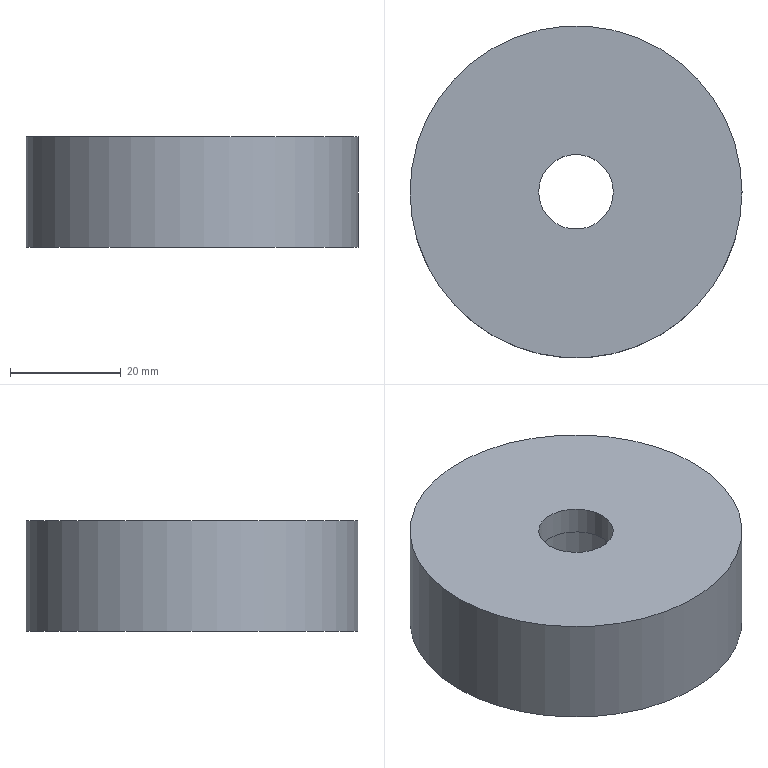Part | NX | features solid 2 | 1 solid | 6 faces | box 60 x 60 x 20 mm | volume 51121 mm3 | cylinder 3 | plane 3 | commonest cylinder face diameters 13.5 x1 20 x1 60 x1
STEP:
#1=CARTESIAN_POINT('',(-260.,-630.,220.));
#2=VERTEX_POINT('',#1);
#3=CARTESIAN_POINT('',(-290.,-630.,220.));
#4=DIRECTION('',(0.,0.,1.));
#5=DIRECTION('',(1.,0.,0.));
#6=AXIS2_PLACEMENT_3D('',#3,#4,#5);
#7=CIRCLE('',#6,30.);
#8=EDGE_CURVE('',#2,#2,#7,.T.);
#9=ORIENTED_EDGE('',*,*,#8,.T.);
#10=EDGE_LOOP('',(#9));
#11=FACE_BOUND('',#10,.T.);
#12=CARTESIAN_POINT('',(-260.,-630.,240.));
#13=VERTEX_POINT('',#12);
#14=CARTESIAN_POINT('',(-290.,-630.,240.));
#15=DIRECTION('',(0.,0.,1.));
#16=DIRECTION('',(1.,0.,0.));
#17=AXIS2_PLACEMENT_3D('',#14,#15,#16);
#18=CIRCLE('',#17,30.);
#19=EDGE_CURVE('',#13,#13,#18,.T.);
#20=ORIENTED_EDGE('',*,*,#19,.F.);
#21=EDGE_LOOP('',(#20));
#22=FACE_BOUND('',#21,.T.);
#23=CARTESIAN_POINT('',(-290.,-630.,220.));
#24=DIRECTION('',(0.,0.,1.));
#25=DIRECTION('',(-1.,0.,0.));
#26=AXIS2_PLACEMENT_3D('',#23,#24,#25);
#27=CYLINDRICAL_SURFACE('',#26,30.);
#28=ADVANCED_FACE('',(#11,#22),#27,.T.);
#29=CARTESIAN_POINT('',(-280.,-630.,220.));
#30=VERTEX_POINT('',#29);
#31=CARTESIAN_POINT('',(-290.,-630.,220.));
#32=DIRECTION('',(0.,0.,1.));
#33=DIRECTION('',(1.,0.,0.));
#34=AXIS2_PLACEMENT_3D('',#31,#32,#33);
#35=CIRCLE('',#34,10.);
#36=EDGE_CURVE('',#30,#30,#35,.T.);
#37=ORIENTED_EDGE('',*,*,#36,.T.);
#38=EDGE_LOOP('',(#37));
#39=FACE_BOUND('',#38,.T.);
#40=ORIENTED_EDGE('',*,*,#8,.F.);
#41=EDGE_LOOP('',(#40));
#42=FACE_BOUND('',#41,.T.);
#43=CARTESIAN_POINT('',(85.,-1843.22,220.));
#44=DIRECTION('',(0.,0.,-1.));
#45=DIRECTION('',(1.,0.,0.));
#46=AXIS2_PLACEMENT_3D('',#43,#44,#45);
#47=PLANE('',#46);
#48=ADVANCED_FACE('',(#39,#42),#47,.T.);
#49=CARTESIAN_POINT('',(-296.75,-630.,240.));
#50=VERTEX_POINT('',#49);
#51=CARTESIAN_POINT('',(-290.,-630.,240.));
#52=DIRECTION('',(0.,0.,-1.));
#53=DIRECTION('',(-1.,0.,0.));
#54=AXIS2_PLACEMENT_3D('',#51,#52,#53);
#55=CIRCLE('',#54,6.75);
#56=EDGE_CURVE('',#50,#50,#55,.F.);
#57=ORIENTED_EDGE('',*,*,#56,.F.);
#58=EDGE_LOOP('',(#57));
#59=FACE_BOUND('',#58,.T.);
#60=ORIENTED_EDGE('',*,*,#19,.T.);
#61=EDGE_LOOP('',(#60));
#62=FACE_BOUND('',#61,.T.);
#63=CARTESIAN_POINT('',(85.,-1843.22,240.));
#64=DIRECTION('',(0.,0.,-1.));
#65=DIRECTION('',(1.,0.,0.));
#66=AXIS2_PLACEMENT_3D('',#63,#64,#65);
#67=PLANE('',#66);
#68=ADVANCED_FACE('',(#59,#62),#67,.F.);
#69=ORIENTED_EDGE('',*,*,#56,.T.);
#70=EDGE_LOOP('',(#69));
#71=FACE_BOUND('',#70,.T.);
#72=CARTESIAN_POINT('',(-283.25,-630.,235.));
#73=VERTEX_POINT('',#72);
#74=CARTESIAN_POINT('',(-290.,-630.,235.));
#75=DIRECTION('',(0.,0.,1.));
#76=DIRECTION('',(1.,0.,0.));
#77=AXIS2_PLACEMENT_3D('',#74,#75,#76);
#78=CIRCLE('',#77,6.75);
#79=EDGE_CURVE('',#73,#73,#78,.T.);
#80=ORIENTED_EDGE('',*,*,#79,.F.);
#81=EDGE_LOOP('',(#80));
#82=FACE_BOUND('',#81,.T.);
#83=CARTESIAN_POINT('',(-290.,-630.,270.));
#84=DIRECTION('',(0.,0.,1.));
#85=DIRECTION('',(1.,0.,0.));
#86=AXIS2_PLACEMENT_3D('',#83,#84,#85);
#87=CYLINDRICAL_SURFACE('',#86,6.75);
#88=ADVANCED_FACE('',(#71,#82),#87,.F.);
#89=ORIENTED_EDGE('',*,*,#79,.T.);
#90=EDGE_LOOP('',(#89));
#91=FACE_BOUND('',#90,.T.);
#92=CARTESIAN_POINT('',(-280.,-630.,235.));
#93=VERTEX_POINT('',#92);
#94=CARTESIAN_POINT('',(-290.,-630.,235.));
#95=DIRECTION('',(0.,0.,1.));
#96=DIRECTION('',(1.,0.,0.));
#97=AXIS2_PLACEMENT_3D('',#94,#95,#96);
#98=CIRCLE('',#97,10.);
#99=EDGE_CURVE('',#93,#93,#98,.T.);
#100=ORIENTED_EDGE('',*,*,#99,.F.);
#101=EDGE_LOOP('',(#100));
#102=FACE_BOUND('',#101,.T.);
#103=CARTESIAN_POINT('',(-290.,-630.,235.));
#104=DIRECTION('',(0.,0.,1.));
#105=DIRECTION('',(1.,0.,0.));
#106=AXIS2_PLACEMENT_3D('',#103,#104,#105);
#107=PLANE('',#106);
#108=ADVANCED_FACE('',(#91,#102),#107,.F.);
#109=ORIENTED_EDGE('',*,*,#99,.T.);
#110=EDGE_LOOP('',(#109));
#111=FACE_BOUND('',#110,.T.);
#112=ORIENTED_EDGE('',*,*,#36,.F.);
#113=EDGE_LOOP('',(#112));
#114=FACE_BOUND('',#113,.T.);
#115=CARTESIAN_POINT('',(-290.,-630.,220.));
#116=DIRECTION('',(0.,0.,1.));
#117=DIRECTION('',(1.,0.,0.));
#118=AXIS2_PLACEMENT_3D('',#115,#116,#117);
#119=CYLINDRICAL_SURFACE('',#118,10.);
#120=ADVANCED_FACE('',(#111,#114),#119,.F.);
#121=CLOSED_SHELL('',(#28,#48,#68,#88,#108,#120));
#122=MANIFOLD_SOLID_BREP('',#121);
#123=(LENGTH_UNIT()NAMED_UNIT(*)SI_UNIT(.MILLI.,.METRE.));
#124=UNCERTAINTY_MEASURE_WITH_UNIT(LENGTH_MEASURE(0.00001),#123,'','');
#125=(NAMED_UNIT(*)PLANE_ANGLE_UNIT()SI_UNIT($,.RADIAN.));
#126=(NAMED_UNIT(*)SI_UNIT($,.STERADIAN.)SOLID_ANGLE_UNIT());
#127=(GEOMETRIC_REPRESENTATION_CONTEXT(3)GLOBAL_UNCERTAINTY_ASSIGNED_CONTEXT((#124))GLOBAL_UNIT_ASSIGNED_CONTEXT((#123,#125,#126))REPRESENTATION_CONTEXT('',''));
#128=ADVANCED_BREP_SHAPE_REPRESENTATION('',(#122),#127);